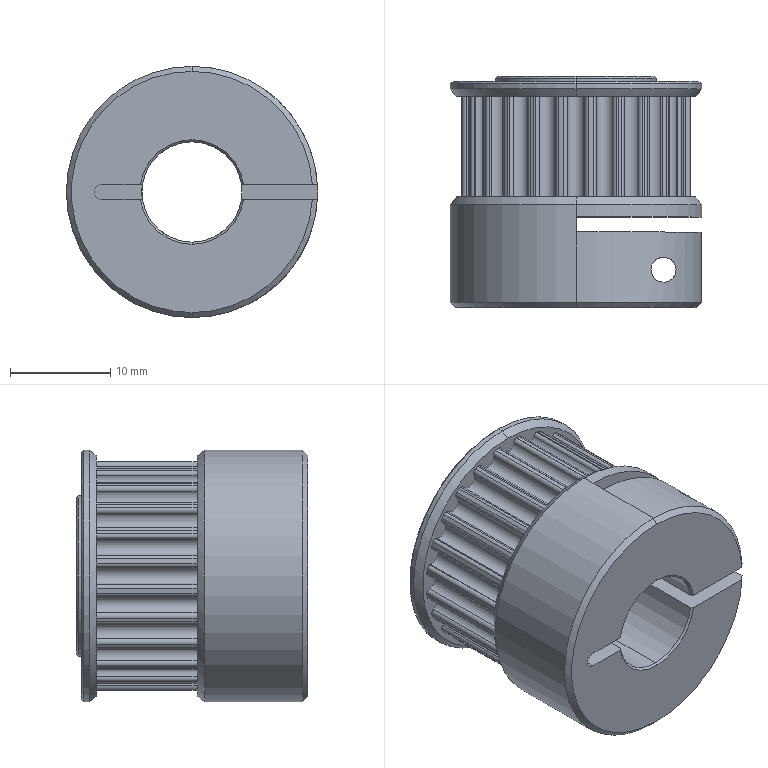Part | STEP file | Timing pulley 24-3M-φ10-23 | 1 solid | 170 faces | box 25 x 23 x 25 mm | volume 7405 mm3 | cylinder 138 | cone 16 | plane 16 | commonest cylinder face diameters 0.8 x60 1.7 x35 22.92 x24 25 x6 10 x4 2.5 x2